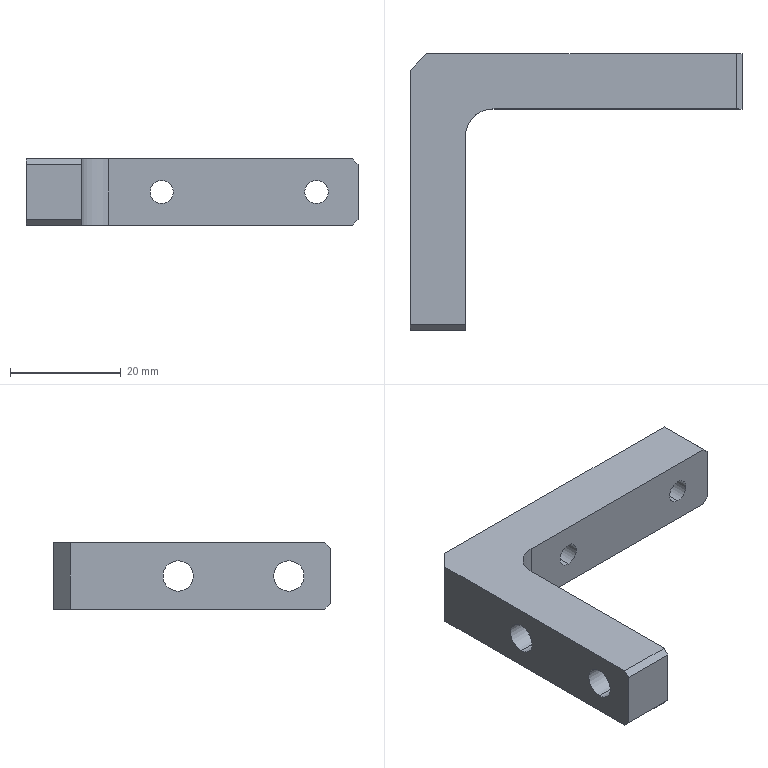Part | SolidWorks | features HoleWzd 2, Chamfer 1, Extrusion 1, Fillet 1 | 1 solid | 22 faces | box 60 x 50 x 12 mm | volume 11238 mm3 | plane 13 | cylinder 9 | commonest cylinder face diameters 4.2 x4 5.5 x4 10 x1
STEP:
#1=CARTESIAN_POINT('',(0.,-42.5,8.75));
#2=VERTEX_POINT('',#1);
#3=CARTESIAN_POINT('',(0.,-42.5,3.25));
#4=VERTEX_POINT('',#3);
#5=CARTESIAN_POINT('',(0.,-42.5,6.));
#6=DIRECTION('',(1.,0.,0.));
#7=DIRECTION('',(0.,0.,-1.));
#8=AXIS2_PLACEMENT_3D('',#5,#6,#7);
#9=CIRCLE('',#8,2.75);
#10=EDGE_CURVE('',#2,#4,#9,.T.);
#11=ORIENTED_EDGE('',*,*,#10,.F.);
#12=CARTESIAN_POINT('',(10.,-42.5,8.75));
#13=VERTEX_POINT('',#12);
#14=CARTESIAN_POINT('',(10.,-42.5,8.75));
#15=DIRECTION('',(1.,0.,0.));
#16=VECTOR('',#15,1000.);
#17=LINE('',#14,#16);
#18=EDGE_CURVE('',#2,#13,#17,.T.);
#19=ORIENTED_EDGE('',*,*,#18,.T.);
#20=CARTESIAN_POINT('',(10.,-42.5,3.25));
#21=VERTEX_POINT('',#20);
#22=CARTESIAN_POINT('',(10.,-42.5,6.));
#23=DIRECTION('',(1.,0.,0.));
#24=DIRECTION('',(0.,0.,-1.));
#25=AXIS2_PLACEMENT_3D('',#22,#23,#24);
#26=CIRCLE('',#25,2.75);
#27=EDGE_CURVE('',#13,#21,#26,.T.);
#28=ORIENTED_EDGE('',*,*,#27,.T.);
#29=CARTESIAN_POINT('',(10.,-42.5,3.25));
#30=DIRECTION('',(1.,0.,0.));
#31=VECTOR('',#30,1000.);
#32=LINE('',#29,#31);
#33=EDGE_CURVE('',#4,#21,#32,.T.);
#34=ORIENTED_EDGE('',*,*,#33,.F.);
#35=EDGE_LOOP('',(#11,#19,#28,#34));
#36=FACE_OUTER_BOUND('',#35,.T.);
#37=CARTESIAN_POINT('',(10.,-42.5,6.));
#38=DIRECTION('',(1.,0.,0.));
#39=DIRECTION('',(0.,0.,-1.));
#40=AXIS2_PLACEMENT_3D('',#37,#38,#39);
#41=CYLINDRICAL_SURFACE('',#40,2.75);
#42=ADVANCED_FACE('',(#36),#41,.F.);
#43=CARTESIAN_POINT('',(0.,-22.5,8.75));
#44=VERTEX_POINT('',#43);
#45=CARTESIAN_POINT('',(0.,-22.5,3.25));
#46=VERTEX_POINT('',#45);
#47=CARTESIAN_POINT('',(0.,-22.5,6.));
#48=DIRECTION('',(1.,0.,0.));
#49=DIRECTION('',(0.,0.,-1.));
#50=AXIS2_PLACEMENT_3D('',#47,#48,#49);
#51=CIRCLE('',#50,2.75);
#52=EDGE_CURVE('',#44,#46,#51,.T.);
#53=ORIENTED_EDGE('',*,*,#52,.F.);
#54=CARTESIAN_POINT('',(10.,-22.5,8.75));
#55=VERTEX_POINT('',#54);
#56=CARTESIAN_POINT('',(10.,-22.5,8.75));
#57=DIRECTION('',(1.,0.,0.));
#58=VECTOR('',#57,1000.);
#59=LINE('',#56,#58);
#60=EDGE_CURVE('',#44,#55,#59,.T.);
#61=ORIENTED_EDGE('',*,*,#60,.T.);
#62=CARTESIAN_POINT('',(10.,-22.5,3.25));
#63=VERTEX_POINT('',#62);
#64=CARTESIAN_POINT('',(10.,-22.5,6.));
#65=DIRECTION('',(1.,0.,0.));
#66=DIRECTION('',(0.,0.,-1.));
#67=AXIS2_PLACEMENT_3D('',#64,#65,#66);
#68=CIRCLE('',#67,2.75);
#69=EDGE_CURVE('',#55,#63,#68,.T.);
#70=ORIENTED_EDGE('',*,*,#69,.T.);
#71=CARTESIAN_POINT('',(10.,-22.5,3.25));
#72=DIRECTION('',(1.,0.,0.));
#73=VECTOR('',#72,1000.);
#74=LINE('',#71,#73);
#75=EDGE_CURVE('',#46,#63,#74,.T.);
#76=ORIENTED_EDGE('',*,*,#75,.F.);
#77=EDGE_LOOP('',(#53,#61,#70,#76));
#78=FACE_OUTER_BOUND('',#77,.T.);
#79=CARTESIAN_POINT('',(10.,-22.5,6.));
#80=DIRECTION('',(1.,0.,0.));
#81=DIRECTION('',(0.,0.,-1.));
#82=AXIS2_PLACEMENT_3D('',#79,#80,#81);
#83=CYLINDRICAL_SURFACE('',#82,2.75);
#84=ADVANCED_FACE('',(#78),#83,.F.);
#85=CARTESIAN_POINT('',(52.5,-10.,3.9));
#86=VERTEX_POINT('',#85);
#87=CARTESIAN_POINT('',(52.5,-10.,8.1));
#88=VERTEX_POINT('',#87);
#89=CARTESIAN_POINT('',(52.5,-10.,6.));
#90=DIRECTION('',(0.,1.,0.));
#91=DIRECTION('',(0.,0.,1.));
#92=AXIS2_PLACEMENT_3D('',#89,#90,#91);
#93=CIRCLE('',#92,2.1);
#94=EDGE_CURVE('',#86,#88,#93,.T.);
#95=ORIENTED_EDGE('',*,*,#94,.F.);
#96=CARTESIAN_POINT('',(52.5,0.,3.9));
#97=VERTEX_POINT('',#96);
#98=CARTESIAN_POINT('',(52.5,0.,3.9));
#99=DIRECTION('',(0.,1.,0.));
#100=VECTOR('',#99,1000.);
#101=LINE('',#98,#100);
#102=EDGE_CURVE('',#86,#97,#101,.T.);
#103=ORIENTED_EDGE('',*,*,#102,.T.);
#104=CARTESIAN_POINT('',(52.5,0.,8.1));
#105=VERTEX_POINT('',#104);
#106=CARTESIAN_POINT('',(52.5,0.,6.));
#107=DIRECTION('',(0.,1.,0.));
#108=DIRECTION('',(0.,0.,1.));
#109=AXIS2_PLACEMENT_3D('',#106,#107,#108);
#110=CIRCLE('',#109,2.1);
#111=EDGE_CURVE('',#97,#105,#110,.T.);
#112=ORIENTED_EDGE('',*,*,#111,.T.);
#113=CARTESIAN_POINT('',(52.5,0.,8.1));
#114=DIRECTION('',(0.,1.,0.));
#115=VECTOR('',#114,1000.);
#116=LINE('',#113,#115);
#117=EDGE_CURVE('',#88,#105,#116,.T.);
#118=ORIENTED_EDGE('',*,*,#117,.F.);
#119=EDGE_LOOP('',(#95,#103,#112,#118));
#120=FACE_OUTER_BOUND('',#119,.T.);
#121=CARTESIAN_POINT('',(52.5,0.,6.));
#122=DIRECTION('',(0.,1.,0.));
#123=DIRECTION('',(0.,0.,1.));
#124=AXIS2_PLACEMENT_3D('',#121,#122,#123);
#125=CYLINDRICAL_SURFACE('',#124,2.1);
#126=ADVANCED_FACE('',(#120),#125,.F.);
#127=CARTESIAN_POINT('',(24.5,-10.,3.9));
#128=VERTEX_POINT('',#127);
#129=CARTESIAN_POINT('',(24.5,-10.,8.1));
#130=VERTEX_POINT('',#129);
#131=CARTESIAN_POINT('',(24.5,-10.,6.));
#132=DIRECTION('',(0.,1.,0.));
#133=DIRECTION('',(0.,0.,1.));
#134=AXIS2_PLACEMENT_3D('',#131,#132,#133);
#135=CIRCLE('',#134,2.1);
#136=EDGE_CURVE('',#128,#130,#135,.T.);
#137=ORIENTED_EDGE('',*,*,#136,.F.);
#138=CARTESIAN_POINT('',(24.5,0.,3.9));
#139=VERTEX_POINT('',#138);
#140=CARTESIAN_POINT('',(24.5,0.,3.9));
#141=DIRECTION('',(0.,1.,0.));
#142=VECTOR('',#141,1000.);
#143=LINE('',#140,#142);
#144=EDGE_CURVE('',#128,#139,#143,.T.);
#145=ORIENTED_EDGE('',*,*,#144,.T.);
#146=CARTESIAN_POINT('',(24.5,0.,8.1));
#147=VERTEX_POINT('',#146);
#148=CARTESIAN_POINT('',(24.5,0.,6.));
#149=DIRECTION('',(0.,1.,0.));
#150=DIRECTION('',(0.,0.,1.));
#151=AXIS2_PLACEMENT_3D('',#148,#149,#150);
#152=CIRCLE('',#151,2.1);
#153=EDGE_CURVE('',#139,#147,#152,.T.);
#154=ORIENTED_EDGE('',*,*,#153,.T.);
#155=CARTESIAN_POINT('',(24.5,0.,8.1));
#156=DIRECTION('',(0.,1.,0.));
#157=VECTOR('',#156,1000.);
#158=LINE('',#155,#157);
#159=EDGE_CURVE('',#130,#147,#158,.T.);
#160=ORIENTED_EDGE('',*,*,#159,.F.);
#161=EDGE_LOOP('',(#137,#145,#154,#160));
#162=FACE_OUTER_BOUND('',#161,.T.);
#163=CARTESIAN_POINT('',(24.5,0.,6.));
#164=DIRECTION('',(0.,1.,0.));
#165=DIRECTION('',(0.,0.,1.));
#166=AXIS2_PLACEMENT_3D('',#163,#164,#165);
#167=CYLINDRICAL_SURFACE('',#166,2.1);
#168=ADVANCED_FACE('',(#162),#167,.F.);
#169=CARTESIAN_POINT('',(60.,0.,11.));
#170=VERTEX_POINT('',#169);
#171=CARTESIAN_POINT('',(60.,0.,1.));
#172=VERTEX_POINT('',#171);
#173=CARTESIAN_POINT('',(60.,0.,12.));
#174=DIRECTION('',(0.,0.,-1.));
#175=VECTOR('',#174,1000.);
#176=LINE('',#173,#175);
#177=EDGE_CURVE('',#170,#172,#176,.T.);
#178=ORIENTED_EDGE('',*,*,#177,.F.);
#179=CARTESIAN_POINT('',(60.,-10.,11.));
#180=VERTEX_POINT('',#179);
#181=CARTESIAN_POINT('',(60.,-10.,11.));
#182=DIRECTION('',(0.,-1.,0.));
#183=VECTOR('',#182,1000.);
#184=LINE('',#181,#183);
#185=EDGE_CURVE('',#170,#180,#184,.T.);
#186=ORIENTED_EDGE('',*,*,#185,.T.);
#187=CARTESIAN_POINT('',(60.,-10.,1.));
#188=VERTEX_POINT('',#187);
#189=CARTESIAN_POINT('',(60.,-10.,12.));
#190=DIRECTION('',(0.,0.,-1.));
#191=VECTOR('',#190,1000.);
#192=LINE('',#189,#191);
#193=EDGE_CURVE('',#180,#188,#192,.T.);
#194=ORIENTED_EDGE('',*,*,#193,.T.);
#195=CARTESIAN_POINT('',(60.,0.,1.));
#196=DIRECTION('',(0.,1.,0.));
#197=VECTOR('',#196,1000.);
#198=LINE('',#195,#197);
#199=EDGE_CURVE('',#188,#172,#198,.T.);
#200=ORIENTED_EDGE('',*,*,#199,.T.);
#201=EDGE_LOOP('',(#178,#186,#194,#200));
#202=FACE_OUTER_BOUND('',#201,.T.);
#203=CARTESIAN_POINT('',(60.,-10.,12.));
#204=DIRECTION('',(-1.,0.,0.));
#205=DIRECTION('',(0.,0.,1.));
#206=AXIS2_PLACEMENT_3D('',#203,#204,#205);
#207=PLANE('',#206);
#208=ADVANCED_FACE('',(#202),#207,.F.);
#209=CARTESIAN_POINT('',(52.5,0.,6.));
#210=DIRECTION('',(0.,1.,0.));
#211=DIRECTION('',(0.,0.,1.));
#212=AXIS2_PLACEMENT_3D('',#209,#210,#211);
#213=CIRCLE('',#212,2.1);
#214=EDGE_CURVE('',#105,#97,#213,.T.);
#215=ORIENTED_EDGE('',*,*,#214,.F.);
#216=ORIENTED_EDGE('',*,*,#111,.F.);
#217=EDGE_LOOP('',(#215,#216));
#218=FACE_BOUND('',#217,.T.);
#219=CARTESIAN_POINT('',(24.5,0.,6.));
#220=DIRECTION('',(0.,1.,0.));
#221=DIRECTION('',(0.,0.,1.));
#222=AXIS2_PLACEMENT_3D('',#219,#220,#221);
#223=CIRCLE('',#222,2.1);
#224=EDGE_CURVE('',#147,#139,#223,.T.);
#225=ORIENTED_EDGE('',*,*,#224,.F.);
#226=ORIENTED_EDGE('',*,*,#153,.F.);
#227=EDGE_LOOP('',(#225,#226));
#228=FACE_BOUND('',#227,.T.);
#229=CARTESIAN_POINT('',(59.,0.,12.));
#230=VERTEX_POINT('',#229);
#231=CARTESIAN_POINT('',(3.,0.,12.));
#232=VERTEX_POINT('',#231);
#233=CARTESIAN_POINT('',(3.,0.,12.));
#234=DIRECTION('',(-1.,0.,0.));
#235=VECTOR('',#234,1000.);
#236=LINE('',#233,#235);
#237=EDGE_CURVE('',#230,#232,#236,.T.);
#238=ORIENTED_EDGE('',*,*,#237,.F.);
#239=CARTESIAN_POINT('',(59.,0.,12.));
#240=DIRECTION('',(0.7071,0.,-0.7071));
#241=VECTOR('',#240,1000.);
#242=LINE('',#239,#241);
#243=EDGE_CURVE('',#230,#170,#242,.T.);
#244=ORIENTED_EDGE('',*,*,#243,.T.);
#245=ORIENTED_EDGE('',*,*,#177,.T.);
#246=CARTESIAN_POINT('',(59.,0.,0.));
#247=VERTEX_POINT('',#246);
#248=CARTESIAN_POINT('',(60.,0.,1.));
#249=DIRECTION('',(-0.7071,0.,-0.7071));
#250=VECTOR('',#249,1000.);
#251=LINE('',#248,#250);
#252=EDGE_CURVE('',#172,#247,#251,.T.);
#253=ORIENTED_EDGE('',*,*,#252,.T.);
#254=CARTESIAN_POINT('',(3.,0.,0.));
#255=VERTEX_POINT('',#254);
#256=CARTESIAN_POINT('',(3.,0.,0.));
#257=DIRECTION('',(-1.,0.,0.));
#258=VECTOR('',#257,1000.);
#259=LINE('',#256,#258);
#260=EDGE_CURVE('',#247,#255,#259,.T.);
#261=ORIENTED_EDGE('',*,*,#260,.T.);
#262=CARTESIAN_POINT('',(3.,0.,12.));
#263=DIRECTION('',(0.,0.,-1.));
#264=VECTOR('',#263,1000.);
#265=LINE('',#262,#264);
#266=EDGE_CURVE('',#232,#255,#265,.T.);
#267=ORIENTED_EDGE('',*,*,#266,.F.);
#268=EDGE_LOOP('',(#238,#244,#245,#253,#261,#267));
#269=FACE_OUTER_BOUND('',#268,.T.);
#270=CARTESIAN_POINT('',(3.,0.,12.));
#271=DIRECTION('',(0.,-1.,0.));
#272=DIRECTION('',(0.,0.,-1.));
#273=AXIS2_PLACEMENT_3D('',#270,#271,#272);
#274=PLANE('',#273);
#275=ADVANCED_FACE('',(#218,#228,#269),#274,.F.);
#276=CARTESIAN_POINT('',(0.,-3.,0.));
#277=VERTEX_POINT('',#276);
#278=CARTESIAN_POINT('',(3.,0.,0.));
#279=DIRECTION('',(-0.7071,-0.7071,0.));
#280=VECTOR('',#279,1000.);
#281=LINE('',#278,#280);
#282=EDGE_CURVE('',#255,#277,#281,.T.);
#283=ORIENTED_EDGE('',*,*,#282,.T.);
#284=CARTESIAN_POINT('',(0.,-3.,12.));
#285=VERTEX_POINT('',#284);
#286=CARTESIAN_POINT('',(0.,-3.,12.));
#287=DIRECTION('',(0.,0.,-1.));
#288=VECTOR('',#287,1000.);
#289=LINE('',#286,#288);
#290=EDGE_CURVE('',#285,#277,#289,.T.);
#291=ORIENTED_EDGE('',*,*,#290,.F.);
#292=CARTESIAN_POINT('',(3.,0.,12.));
#293=DIRECTION('',(-0.7071,-0.7071,0.));
#294=VECTOR('',#293,1000.);
#295=LINE('',#292,#294);
#296=EDGE_CURVE('',#232,#285,#295,.T.);
#297=ORIENTED_EDGE('',*,*,#296,.F.);
#298=ORIENTED_EDGE('',*,*,#266,.T.);
#299=EDGE_LOOP('',(#283,#291,#297,#298));
#300=FACE_OUTER_BOUND('',#299,.T.);
#301=CARTESIAN_POINT('',(3.,0.,12.));
#302=DIRECTION('',(0.7071,-0.7071,0.));
#303=DIRECTION('',(0.7071,0.7071,0.));
#304=AXIS2_PLACEMENT_3D('',#301,#302,#303);
#305=PLANE('',#304);
#306=ADVANCED_FACE('',(#300),#305,.F.);
#307=CARTESIAN_POINT('',(0.,-42.5,6.));
#308=DIRECTION('',(1.,0.,0.));
#309=DIRECTION('',(0.,0.,-1.));
#310=AXIS2_PLACEMENT_3D('',#307,#308,#309);
#311=CIRCLE('',#310,2.75);
#312=EDGE_CURVE('',#4,#2,#311,.T.);
#313=ORIENTED_EDGE('',*,*,#312,.T.);
#314=ORIENTED_EDGE('',*,*,#10,.T.);
#315=EDGE_LOOP('',(#313,#314));
#316=FACE_BOUND('',#315,.T.);
#317=CARTESIAN_POINT('',(0.,-22.5,6.));
#318=DIRECTION('',(1.,0.,0.));
#319=DIRECTION('',(0.,0.,-1.));
#320=AXIS2_PLACEMENT_3D('',#317,#318,#319);
#321=CIRCLE('',#320,2.75);
#322=EDGE_CURVE('',#46,#44,#321,.T.);
#323=ORIENTED_EDGE('',*,*,#322,.T.);
#324=ORIENTED_EDGE('',*,*,#52,.T.);
#325=EDGE_LOOP('',(#323,#324));
#326=FACE_BOUND('',#325,.T.);
#327=CARTESIAN_POINT('',(0.,-50.,11.));
#328=VERTEX_POINT('',#327);
#329=CARTESIAN_POINT('',(0.,-50.,1.));
#330=VERTEX_POINT('',#329);
#331=CARTESIAN_POINT('',(0.,-50.,12.));
#332=DIRECTION('',(0.,0.,-1.));
#333=VECTOR('',#332,1000.);
#334=LINE('',#331,#333);
#335=EDGE_CURVE('',#328,#330,#334,.T.);
#336=ORIENTED_EDGE('',*,*,#335,.F.);
#337=CARTESIAN_POINT('',(0.,-49.,12.));
#338=VERTEX_POINT('',#337);
#339=CARTESIAN_POINT('',(0.,-49.,12.));
#340=DIRECTION('',(0.,0.7071,0.7071));
#341=VECTOR('',#340,1000.);
#342=LINE('',#339,#341);
#343=EDGE_CURVE('',#328,#338,#342,.T.);
#344=ORIENTED_EDGE('',*,*,#343,.T.);
#345=CARTESIAN_POINT('',(0.,-50.,12.));
#346=DIRECTION('',(0.,-1.,0.));
#347=VECTOR('',#346,1000.);
#348=LINE('',#345,#347);
#349=EDGE_CURVE('',#285,#338,#348,.T.);
#350=ORIENTED_EDGE('',*,*,#349,.F.);
#351=ORIENTED_EDGE('',*,*,#290,.T.);
#352=CARTESIAN_POINT('',(0.,-49.,0.));
#353=VERTEX_POINT('',#352);
#354=CARTESIAN_POINT('',(0.,-50.,0.));
#355=DIRECTION('',(0.,-1.,0.));
#356=VECTOR('',#355,1000.);
#357=LINE('',#354,#356);
#358=EDGE_CURVE('',#277,#353,#357,.T.);
#359=ORIENTED_EDGE('',*,*,#358,.T.);
#360=CARTESIAN_POINT('',(0.,-50.,1.));
#361=DIRECTION('',(0.,-0.7071,0.7071));
#362=VECTOR('',#361,1000.);
#363=LINE('',#360,#362);
#364=EDGE_CURVE('',#353,#330,#363,.T.);
#365=ORIENTED_EDGE('',*,*,#364,.T.);
#366=EDGE_LOOP('',(#336,#344,#350,#351,#359,#365));
#367=FACE_OUTER_BOUND('',#366,.T.);
#368=CARTESIAN_POINT('',(0.,-50.,12.));
#369=DIRECTION('',(1.,0.,0.));
#370=DIRECTION('',(0.,0.,-1.));
#371=AXIS2_PLACEMENT_3D('',#368,#369,#370);
#372=PLANE('',#371);
#373=ADVANCED_FACE('',(#316,#326,#367),#372,.F.);
#374=CARTESIAN_POINT('',(10.,-50.,11.));
#375=VERTEX_POINT('',#374);
#376=CARTESIAN_POINT('',(10.,-50.,1.));
#377=VERTEX_POINT('',#376);
#378=CARTESIAN_POINT('',(10.,-50.,12.));
#379=DIRECTION('',(0.,0.,-1.));
#380=VECTOR('',#379,1000.);
#381=LINE('',#378,#380);
#382=EDGE_CURVE('',#375,#377,#381,.T.);
#383=ORIENTED_EDGE('',*,*,#382,.F.);
#384=CARTESIAN_POINT('',(0.,-50.,11.));
#385=DIRECTION('',(-1.,0.,0.));
#386=VECTOR('',#385,1000.);
#387=LINE('',#384,#386);
#388=EDGE_CURVE('',#375,#328,#387,.T.);
#389=ORIENTED_EDGE('',*,*,#388,.T.);
#390=ORIENTED_EDGE('',*,*,#335,.T.);
#391=CARTESIAN_POINT('',(10.,-50.,1.));
#392=DIRECTION('',(1.,0.,0.));
#393=VECTOR('',#392,1000.);
#394=LINE('',#391,#393);
#395=EDGE_CURVE('',#330,#377,#394,.T.);
#396=ORIENTED_EDGE('',*,*,#395,.T.);
#397=EDGE_LOOP('',(#383,#389,#390,#396));
#398=FACE_OUTER_BOUND('',#397,.T.);
#399=CARTESIAN_POINT('',(0.,-50.,12.));
#400=DIRECTION('',(0.,1.,0.));
#401=DIRECTION('',(-1.,0.,0.));
#402=AXIS2_PLACEMENT_3D('',#399,#400,#401);
#403=PLANE('',#402);
#404=ADVANCED_FACE('',(#398),#403,.F.);
#405=CARTESIAN_POINT('',(10.,-42.5,6.));
#406=DIRECTION('',(1.,0.,0.));
#407=DIRECTION('',(0.,0.,-1.));
#408=AXIS2_PLACEMENT_3D('',#405,#406,#407);
#409=CIRCLE('',#408,2.75);
#410=EDGE_CURVE('',#21,#13,#409,.T.);
#411=ORIENTED_EDGE('',*,*,#410,.F.);
#412=ORIENTED_EDGE('',*,*,#27,.F.);
#413=EDGE_LOOP('',(#411,#412));
#414=FACE_BOUND('',#413,.T.);
#415=CARTESIAN_POINT('',(10.,-22.5,6.));
#416=DIRECTION('',(1.,0.,0.));
#417=DIRECTION('',(0.,0.,-1.));
#418=AXIS2_PLACEMENT_3D('',#415,#416,#417);
#419=CIRCLE('',#418,2.75);
#420=EDGE_CURVE('',#63,#55,#419,.T.);
#421=ORIENTED_EDGE('',*,*,#420,.F.);
#422=ORIENTED_EDGE('',*,*,#69,.F.);
#423=EDGE_LOOP('',(#421,#422));
#424=FACE_BOUND('',#423,.T.);
#425=CARTESIAN_POINT('',(10.,-49.,0.));
#426=VERTEX_POINT('',#425);
#427=CARTESIAN_POINT('',(10.,-15.,0.));
#428=VERTEX_POINT('',#427);
#429=CARTESIAN_POINT('',(10.,-50.,0.));
#430=DIRECTION('',(0.,1.,0.));
#431=VECTOR('',#430,1000.);
#432=LINE('',#429,#431);
#433=EDGE_CURVE('',#426,#428,#432,.T.);
#434=ORIENTED_EDGE('',*,*,#433,.T.);
#435=CARTESIAN_POINT('',(10.,-15.,12.));
#436=VERTEX_POINT('',#435);
#437=CARTESIAN_POINT('',(10.,-15.,12.));
#438=DIRECTION('',(0.,0.,1.));
#439=VECTOR('',#438,1000.);
#440=LINE('',#437,#439);
#441=EDGE_CURVE('',#428,#436,#440,.T.);
#442=ORIENTED_EDGE('',*,*,#441,.T.);
#443=CARTESIAN_POINT('',(10.,-49.,12.));
#444=VERTEX_POINT('',#443);
#445=CARTESIAN_POINT('',(10.,-50.,12.));
#446=DIRECTION('',(0.,1.,0.));
#447=VECTOR('',#446,1000.);
#448=LINE('',#445,#447);
#449=EDGE_CURVE('',#444,#436,#448,.T.);
#450=ORIENTED_EDGE('',*,*,#449,.F.);
#451=CARTESIAN_POINT('',(10.,-49.,12.));
#452=DIRECTION('',(0.,-0.7071,-0.7071));
#453=VECTOR('',#452,1000.);
#454=LINE('',#451,#453);
#455=EDGE_CURVE('',#444,#375,#454,.T.);
#456=ORIENTED_EDGE('',*,*,#455,.T.);
#457=ORIENTED_EDGE('',*,*,#382,.T.);
#458=CARTESIAN_POINT('',(10.,-50.,1.));
#459=DIRECTION('',(0.,0.7071,-0.7071));
#460=VECTOR('',#459,1000.);
#461=LINE('',#458,#460);
#462=EDGE_CURVE('',#377,#426,#461,.T.);
#463=ORIENTED_EDGE('',*,*,#462,.T.);
#464=EDGE_LOOP('',(#434,#442,#450,#456,#457,#463));
#465=FACE_OUTER_BOUND('',#464,.T.);
#466=CARTESIAN_POINT('',(10.,-50.,12.));
#467=DIRECTION('',(-1.,0.,0.));
#468=DIRECTION('',(0.,-1.,0.));
#469=AXIS2_PLACEMENT_3D('',#466,#467,#468);
#470=PLANE('',#469);
#471=ADVANCED_FACE('',(#414,#424,#465),#470,.F.);
#472=CARTESIAN_POINT('',(52.5,-10.,6.));
#473=DIRECTION('',(0.,1.,0.));
#474=DIRECTION('',(0.,0.,1.));
#475=AXIS2_PLACEMENT_3D('',#472,#473,#474);
#476=CIRCLE('',#475,2.1);
#477=EDGE_CURVE('',#88,#86,#476,.T.);
#478=ORIENTED_EDGE('',*,*,#477,.T.);
#479=ORIENTED_EDGE('',*,*,#94,.T.);
#480=EDGE_LOOP('',(#478,#479));
#481=FACE_BOUND('',#480,.T.);
#482=CARTESIAN_POINT('',(24.5,-10.,6.));
#483=DIRECTION('',(0.,1.,0.));
#484=DIRECTION('',(0.,0.,1.));
#485=AXIS2_PLACEMENT_3D('',#482,#483,#484);
#486=CIRCLE('',#485,2.1);
#487=EDGE_CURVE('',#130,#128,#486,.T.);
#488=ORIENTED_EDGE('',*,*,#487,.T.);
#489=ORIENTED_EDGE('',*,*,#136,.T.);
#490=EDGE_LOOP('',(#488,#489));
#491=FACE_BOUND('',#490,.T.);
#492=CARTESIAN_POINT('',(15.,-10.,12.));
#493=VERTEX_POINT('',#492);
#494=CARTESIAN_POINT('',(59.,-10.,12.));
#495=VERTEX_POINT('',#494);
#496=CARTESIAN_POINT('',(10.,-10.,12.));
#497=DIRECTION('',(1.,0.,0.));
#498=VECTOR('',#497,1000.);
#499=LINE('',#496,#498);
#500=EDGE_CURVE('',#493,#495,#499,.T.);
#501=ORIENTED_EDGE('',*,*,#500,.F.);
#502=CARTESIAN_POINT('',(15.,-10.,0.));
#503=VERTEX_POINT('',#502);
#504=CARTESIAN_POINT('',(15.,-10.,0.));
#505=DIRECTION('',(0.,0.,-1.));
#506=VECTOR('',#505,1000.);
#507=LINE('',#504,#506);
#508=EDGE_CURVE('',#493,#503,#507,.T.);
#509=ORIENTED_EDGE('',*,*,#508,.T.);
#510=CARTESIAN_POINT('',(59.,-10.,0.));
#511=VERTEX_POINT('',#510);
#512=CARTESIAN_POINT('',(10.,-10.,0.));
#513=DIRECTION('',(1.,0.,0.));
#514=VECTOR('',#513,1000.);
#515=LINE('',#512,#514);
#516=EDGE_CURVE('',#503,#511,#515,.T.);
#517=ORIENTED_EDGE('',*,*,#516,.T.);
#518=CARTESIAN_POINT('',(60.,-10.,1.));
#519=DIRECTION('',(0.7071,0.,0.7071));
#520=VECTOR('',#519,1000.);
#521=LINE('',#518,#520);
#522=EDGE_CURVE('',#511,#188,#521,.T.);
#523=ORIENTED_EDGE('',*,*,#522,.T.);
#524=ORIENTED_EDGE('',*,*,#193,.F.);
#525=CARTESIAN_POINT('',(59.,-10.,12.));
#526=DIRECTION('',(-0.7071,0.,0.7071));
#527=VECTOR('',#526,1000.);
#528=LINE('',#525,#527);
#529=EDGE_CURVE('',#180,#495,#528,.T.);
#530=ORIENTED_EDGE('',*,*,#529,.T.);
#531=EDGE_LOOP('',(#501,#509,#517,#523,#524,#530));
#532=FACE_OUTER_BOUND('',#531,.T.);
#533=CARTESIAN_POINT('',(10.,-10.,12.));
#534=DIRECTION('',(0.,1.,0.));
#535=DIRECTION('',(0.,0.,1.));
#536=AXIS2_PLACEMENT_3D('',#533,#534,#535);
#537=PLANE('',#536);
#538=ADVANCED_FACE('',(#481,#491,#532),#537,.F.);
#539=ORIENTED_EDGE('',*,*,#349,.T.);
#540=CARTESIAN_POINT('',(0.,-49.,12.));
#541=DIRECTION('',(1.,0.,0.));
#542=VECTOR('',#541,1000.);
#543=LINE('',#540,#542);
#544=EDGE_CURVE('',#338,#444,#543,.T.);
#545=ORIENTED_EDGE('',*,*,#544,.T.);
#546=ORIENTED_EDGE('',*,*,#449,.T.);
#547=CARTESIAN_POINT('',(15.,-15.,12.));
#548=DIRECTION('',(0.,0.,-1.));
#549=DIRECTION('',(-1.,0.,0.));
#550=AXIS2_PLACEMENT_3D('',#547,#548,#549);
#551=CIRCLE('',#550,5.);
#552=EDGE_CURVE('',#436,#493,#551,.T.);
#553=ORIENTED_EDGE('',*,*,#552,.T.);
#554=ORIENTED_EDGE('',*,*,#500,.T.);
#555=CARTESIAN_POINT('',(59.,0.,12.));
#556=DIRECTION('',(0.,1.,0.));
#557=VECTOR('',#556,1000.);
#558=LINE('',#555,#557);
#559=EDGE_CURVE('',#495,#230,#558,.T.);
#560=ORIENTED_EDGE('',*,*,#559,.T.);
#561=ORIENTED_EDGE('',*,*,#237,.T.);
#562=ORIENTED_EDGE('',*,*,#296,.T.);
#563=EDGE_LOOP('',(#539,#545,#546,#553,#554,#560,#561,#562));
#564=FACE_OUTER_BOUND('',#563,.T.);
#565=CARTESIAN_POINT('',(0.,0.,12.));
#566=DIRECTION('',(0.,0.,-1.));
#567=DIRECTION('',(-1.,0.,0.));
#568=AXIS2_PLACEMENT_3D('',#565,#566,#567);
#569=PLANE('',#568);
#570=ADVANCED_FACE('',(#564),#569,.F.);
#571=ORIENTED_EDGE('',*,*,#433,.F.);
#572=CARTESIAN_POINT('',(0.,-49.,0.));
#573=DIRECTION('',(-1.,0.,0.));
#574=VECTOR('',#573,1000.);
#575=LINE('',#572,#574);
#576=EDGE_CURVE('',#426,#353,#575,.T.);
#577=ORIENTED_EDGE('',*,*,#576,.T.);
#578=ORIENTED_EDGE('',*,*,#358,.F.);
#579=ORIENTED_EDGE('',*,*,#282,.F.);
#580=ORIENTED_EDGE('',*,*,#260,.F.);
#581=CARTESIAN_POINT('',(59.,-10.,0.));
#582=DIRECTION('',(0.,-1.,0.));
#583=VECTOR('',#582,1000.);
#584=LINE('',#581,#583);
#585=EDGE_CURVE('',#247,#511,#584,.T.);
#586=ORIENTED_EDGE('',*,*,#585,.T.);
#587=ORIENTED_EDGE('',*,*,#516,.F.);
#588=CARTESIAN_POINT('',(15.,-15.,0.));
#589=DIRECTION('',(0.,0.,1.));
#590=DIRECTION('',(-1.,0.,0.));
#591=AXIS2_PLACEMENT_3D('',#588,#589,#590);
#592=CIRCLE('',#591,5.);
#593=EDGE_CURVE('',#503,#428,#592,.T.);
#594=ORIENTED_EDGE('',*,*,#593,.T.);
#595=EDGE_LOOP('',(#571,#577,#578,#579,#580,#586,#587,#594));
#596=FACE_OUTER_BOUND('',#595,.T.);
#597=CARTESIAN_POINT('',(0.,0.,0.));
#598=DIRECTION('',(0.,0.,-1.));
#599=DIRECTION('',(-1.,0.,0.));
#600=AXIS2_PLACEMENT_3D('',#597,#598,#599);
#601=PLANE('',#600);
#602=ADVANCED_FACE('',(#596),#601,.T.);
#603=ORIENTED_EDGE('',*,*,#144,.F.);
#604=ORIENTED_EDGE('',*,*,#487,.F.);
#605=ORIENTED_EDGE('',*,*,#159,.T.);
#606=ORIENTED_EDGE('',*,*,#224,.T.);
#607=EDGE_LOOP('',(#603,#604,#605,#606));
#608=FACE_OUTER_BOUND('',#607,.T.);
#609=CARTESIAN_POINT('',(24.5,0.,6.));
#610=DIRECTION('',(0.,1.,0.));
#611=DIRECTION('',(0.,0.,1.));
#612=AXIS2_PLACEMENT_3D('',#609,#610,#611);
#613=CYLINDRICAL_SURFACE('',#612,2.1);
#614=ADVANCED_FACE('',(#608),#613,.F.);
#615=ORIENTED_EDGE('',*,*,#102,.F.);
#616=ORIENTED_EDGE('',*,*,#477,.F.);
#617=ORIENTED_EDGE('',*,*,#117,.T.);
#618=ORIENTED_EDGE('',*,*,#214,.T.);
#619=EDGE_LOOP('',(#615,#616,#617,#618));
#620=FACE_OUTER_BOUND('',#619,.T.);
#621=CARTESIAN_POINT('',(52.5,0.,6.));
#622=DIRECTION('',(0.,1.,0.));
#623=DIRECTION('',(0.,0.,1.));
#624=AXIS2_PLACEMENT_3D('',#621,#622,#623);
#625=CYLINDRICAL_SURFACE('',#624,2.1);
#626=ADVANCED_FACE('',(#620),#625,.F.);
#627=ORIENTED_EDGE('',*,*,#60,.F.);
#628=ORIENTED_EDGE('',*,*,#322,.F.);
#629=ORIENTED_EDGE('',*,*,#75,.T.);
#630=ORIENTED_EDGE('',*,*,#420,.T.);
#631=EDGE_LOOP('',(#627,#628,#629,#630));
#632=FACE_OUTER_BOUND('',#631,.T.);
#633=CARTESIAN_POINT('',(10.,-22.5,6.));
#634=DIRECTION('',(1.,0.,0.));
#635=DIRECTION('',(0.,0.,-1.));
#636=AXIS2_PLACEMENT_3D('',#633,#634,#635);
#637=CYLINDRICAL_SURFACE('',#636,2.75);
#638=ADVANCED_FACE('',(#632),#637,.F.);
#639=ORIENTED_EDGE('',*,*,#18,.F.);
#640=ORIENTED_EDGE('',*,*,#312,.F.);
#641=ORIENTED_EDGE('',*,*,#33,.T.);
#642=ORIENTED_EDGE('',*,*,#410,.T.);
#643=EDGE_LOOP('',(#639,#640,#641,#642));
#644=FACE_OUTER_BOUND('',#643,.T.);
#645=CARTESIAN_POINT('',(10.,-42.5,6.));
#646=DIRECTION('',(1.,0.,0.));
#647=DIRECTION('',(0.,0.,-1.));
#648=AXIS2_PLACEMENT_3D('',#645,#646,#647);
#649=CYLINDRICAL_SURFACE('',#648,2.75);
#650=ADVANCED_FACE('',(#644),#649,.F.);
#651=ORIENTED_EDGE('',*,*,#343,.F.);
#652=ORIENTED_EDGE('',*,*,#388,.F.);
#653=ORIENTED_EDGE('',*,*,#455,.F.);
#654=ORIENTED_EDGE('',*,*,#544,.F.);
#655=EDGE_LOOP('',(#651,#652,#653,#654));
#656=FACE_OUTER_BOUND('',#655,.T.);
#657=CARTESIAN_POINT('',(0.,-49.,12.));
#658=DIRECTION('',(0.,0.7071,-0.7071));
#659=DIRECTION('',(1.,0.,0.));
#660=AXIS2_PLACEMENT_3D('',#657,#658,#659);
#661=PLANE('',#660);
#662=ADVANCED_FACE('',(#656),#661,.F.);
#663=ORIENTED_EDGE('',*,*,#364,.F.);
#664=ORIENTED_EDGE('',*,*,#576,.F.);
#665=ORIENTED_EDGE('',*,*,#462,.F.);
#666=ORIENTED_EDGE('',*,*,#395,.F.);
#667=EDGE_LOOP('',(#663,#664,#665,#666));
#668=FACE_OUTER_BOUND('',#667,.T.);
#669=CARTESIAN_POINT('',(0.,-50.,1.));
#670=DIRECTION('',(0.,-0.7071,-0.7071));
#671=DIRECTION('',(-1.,0.,0.));
#672=AXIS2_PLACEMENT_3D('',#669,#670,#671);
#673=PLANE('',#672);
#674=ADVANCED_FACE('',(#668),#673,.T.);
#675=ORIENTED_EDGE('',*,*,#529,.F.);
#676=ORIENTED_EDGE('',*,*,#185,.F.);
#677=ORIENTED_EDGE('',*,*,#243,.F.);
#678=ORIENTED_EDGE('',*,*,#559,.F.);
#679=EDGE_LOOP('',(#675,#676,#677,#678));
#680=FACE_OUTER_BOUND('',#679,.T.);
#681=CARTESIAN_POINT('',(59.,0.,12.));
#682=DIRECTION('',(-0.7071,0.,-0.7071));
#683=DIRECTION('',(0.,1.,0.));
#684=AXIS2_PLACEMENT_3D('',#681,#682,#683);
#685=PLANE('',#684);
#686=ADVANCED_FACE('',(#680),#685,.F.);
#687=ORIENTED_EDGE('',*,*,#522,.F.);
#688=ORIENTED_EDGE('',*,*,#585,.F.);
#689=ORIENTED_EDGE('',*,*,#252,.F.);
#690=ORIENTED_EDGE('',*,*,#199,.F.);
#691=EDGE_LOOP('',(#687,#688,#689,#690));
#692=FACE_OUTER_BOUND('',#691,.T.);
#693=CARTESIAN_POINT('',(60.,-10.,1.));
#694=DIRECTION('',(0.7071,0.,-0.7071));
#695=DIRECTION('',(0.,-1.,0.));
#696=AXIS2_PLACEMENT_3D('',#693,#694,#695);
#697=PLANE('',#696);
#698=ADVANCED_FACE('',(#692),#697,.T.);
#699=ORIENTED_EDGE('',*,*,#552,.F.);
#700=ORIENTED_EDGE('',*,*,#441,.F.);
#701=ORIENTED_EDGE('',*,*,#593,.F.);
#702=ORIENTED_EDGE('',*,*,#508,.F.);
#703=EDGE_LOOP('',(#699,#700,#701,#702));
#704=FACE_OUTER_BOUND('',#703,.T.);
#705=CARTESIAN_POINT('',(15.,-15.,12.));
#706=DIRECTION('',(0.,0.,1.));
#707=DIRECTION('',(1.,0.,0.));
#708=AXIS2_PLACEMENT_3D('',#705,#706,#707);
#709=CYLINDRICAL_SURFACE('',#708,5.);
#710=ADVANCED_FACE('',(#704),#709,.F.);
#711=CLOSED_SHELL('',(#42,#84,#126,#168,#208,#275,#306,#373,#404,#471,#538,#570,#602,#614,#626,#638,#650,#662,#674,#686,#698,#710));
#712=MANIFOLD_SOLID_BREP('',#711);
#713=CARTESIAN_POINT('',(0.,0.,0.));
#714=DIRECTION('',(0.,0.,1.));
#715=DIRECTION('',(1.,0.,0.));
#716=AXIS2_PLACEMENT_3D('',#713,#714,#715);
#717=(LENGTH_UNIT()NAMED_UNIT(*)SI_UNIT(.MILLI.,.METRE.));
#718=UNCERTAINTY_MEASURE_WITH_UNIT(LENGTH_MEASURE(0.00001),#717,'','');
#719=(NAMED_UNIT(*)PLANE_ANGLE_UNIT()SI_UNIT($,.RADIAN.));
#720=(NAMED_UNIT(*)SI_UNIT($,.STERADIAN.)SOLID_ANGLE_UNIT());
#721=(GEOMETRIC_REPRESENTATION_CONTEXT(3)GLOBAL_UNCERTAINTY_ASSIGNED_CONTEXT((#718))GLOBAL_UNIT_ASSIGNED_CONTEXT((#717,#719,#720))REPRESENTATION_CONTEXT('',''));
#722=ADVANCED_BREP_SHAPE_REPRESENTATION('',(#712,#716),#721);